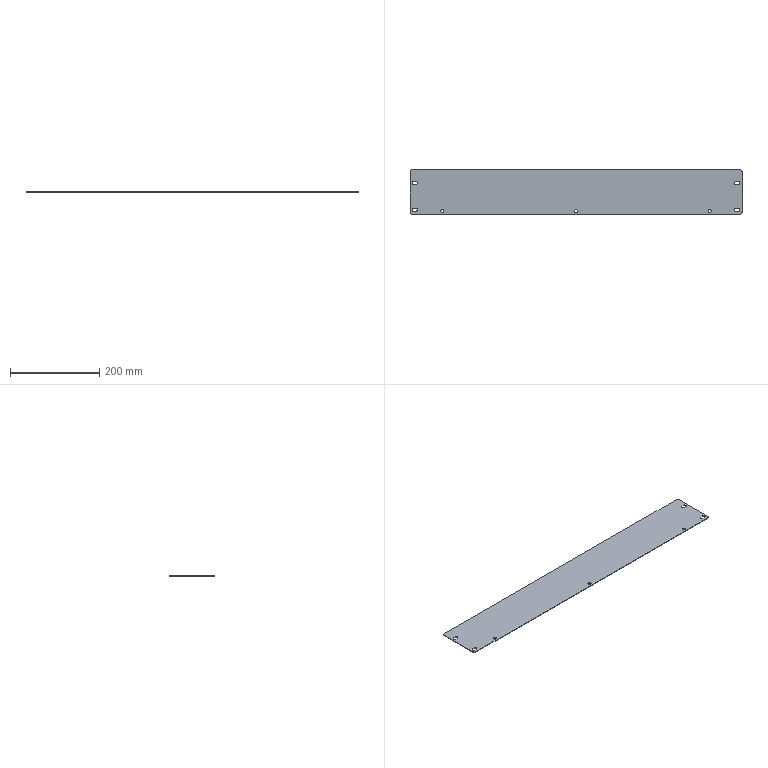Part | SolidWorks | features EdgeFlange 2, Fillet 1, FlatPattern 1, HoleWzd 1, ICE 1, SMBaseFlange 1, SheetMetal 1 | 1 solid | 36 faces | box 745 x 100 x 1.2 mm | volume 88883 mm3 | cylinder 22 | plane 14 | commonest cylinder face diameters 7 x18 10 x4
STEP:
#1=CARTESIAN_POINT('',(303.5,-43.,0.));
#2=VERTEX_POINT('',#1);
#3=CARTESIAN_POINT('',(296.5,-43.,0.));
#4=VERTEX_POINT('',#3);
#5=CARTESIAN_POINT('',(300.,-43.,0.));
#6=DIRECTION('',(0.,0.,-1.));
#7=DIRECTION('',(-1.,0.,0.));
#8=AXIS2_PLACEMENT_3D('',#5,#6,#7);
#9=CIRCLE('',#8,3.5);
#10=EDGE_CURVE('',#2,#4,#9,.T.);
#11=ORIENTED_EDGE('',*,*,#10,.F.);
#12=CARTESIAN_POINT('',(303.5,-43.,-1.2));
#13=VERTEX_POINT('',#12);
#14=CARTESIAN_POINT('',(303.5,-43.,-1.2));
#15=DIRECTION('',(0.,0.,-1.));
#16=VECTOR('',#15,1000.);
#17=LINE('',#14,#16);
#18=EDGE_CURVE('',#2,#13,#17,.T.);
#19=ORIENTED_EDGE('',*,*,#18,.T.);
#20=CARTESIAN_POINT('',(296.5,-43.,-1.2));
#21=VERTEX_POINT('',#20);
#22=CARTESIAN_POINT('',(300.,-43.,-1.2));
#23=DIRECTION('',(0.,0.,-1.));
#24=DIRECTION('',(-1.,0.,0.));
#25=AXIS2_PLACEMENT_3D('',#22,#23,#24);
#26=CIRCLE('',#25,3.5);
#27=EDGE_CURVE('',#13,#21,#26,.T.);
#28=ORIENTED_EDGE('',*,*,#27,.T.);
#29=CARTESIAN_POINT('',(296.5,-43.,-1.2));
#30=DIRECTION('',(0.,0.,-1.));
#31=VECTOR('',#30,1000.);
#32=LINE('',#29,#31);
#33=EDGE_CURVE('',#4,#21,#32,.T.);
#34=ORIENTED_EDGE('',*,*,#33,.F.);
#35=EDGE_LOOP('',(#11,#19,#28,#34));
#36=FACE_OUTER_BOUND('',#35,.T.);
#37=CARTESIAN_POINT('',(300.,-43.,-1.2));
#38=DIRECTION('',(0.,0.,-1.));
#39=DIRECTION('',(-1.,0.,0.));
#40=AXIS2_PLACEMENT_3D('',#37,#38,#39);
#41=CYLINDRICAL_SURFACE('',#40,3.5);
#42=ADVANCED_FACE('',(#36),#41,.F.);
#43=CARTESIAN_POINT('',(3.5,-43.,0.));
#44=VERTEX_POINT('',#43);
#45=CARTESIAN_POINT('',(-3.5,-43.,0.));
#46=VERTEX_POINT('',#45);
#47=CARTESIAN_POINT('',(0.,-43.,0.));
#48=DIRECTION('',(0.,0.,-1.));
#49=DIRECTION('',(-1.,0.,0.));
#50=AXIS2_PLACEMENT_3D('',#47,#48,#49);
#51=CIRCLE('',#50,3.5);
#52=EDGE_CURVE('',#44,#46,#51,.T.);
#53=ORIENTED_EDGE('',*,*,#52,.F.);
#54=CARTESIAN_POINT('',(3.5,-43.,-1.2));
#55=VERTEX_POINT('',#54);
#56=CARTESIAN_POINT('',(3.5,-43.,-1.2));
#57=DIRECTION('',(0.,0.,-1.));
#58=VECTOR('',#57,1000.);
#59=LINE('',#56,#58);
#60=EDGE_CURVE('',#44,#55,#59,.T.);
#61=ORIENTED_EDGE('',*,*,#60,.T.);
#62=CARTESIAN_POINT('',(-3.5,-43.,-1.2));
#63=VERTEX_POINT('',#62);
#64=CARTESIAN_POINT('',(0.,-43.,-1.2));
#65=DIRECTION('',(0.,0.,-1.));
#66=DIRECTION('',(-1.,0.,0.));
#67=AXIS2_PLACEMENT_3D('',#64,#65,#66);
#68=CIRCLE('',#67,3.5);
#69=EDGE_CURVE('',#55,#63,#68,.T.);
#70=ORIENTED_EDGE('',*,*,#69,.T.);
#71=CARTESIAN_POINT('',(-3.5,-43.,-1.2));
#72=DIRECTION('',(0.,0.,-1.));
#73=VECTOR('',#72,1000.);
#74=LINE('',#71,#73);
#75=EDGE_CURVE('',#46,#63,#74,.T.);
#76=ORIENTED_EDGE('',*,*,#75,.F.);
#77=EDGE_LOOP('',(#53,#61,#70,#76));
#78=FACE_OUTER_BOUND('',#77,.T.);
#79=CARTESIAN_POINT('',(0.,-43.,-1.2));
#80=DIRECTION('',(0.,0.,-1.));
#81=DIRECTION('',(-1.,0.,0.));
#82=AXIS2_PLACEMENT_3D('',#79,#80,#81);
#83=CYLINDRICAL_SURFACE('',#82,3.5);
#84=ADVANCED_FACE('',(#78),#83,.F.);
#85=CARTESIAN_POINT('',(-296.5,-43.,0.));
#86=VERTEX_POINT('',#85);
#87=CARTESIAN_POINT('',(-303.5,-43.,0.));
#88=VERTEX_POINT('',#87);
#89=CARTESIAN_POINT('',(-300.,-43.,0.));
#90=DIRECTION('',(0.,0.,-1.));
#91=DIRECTION('',(-1.,0.,0.));
#92=AXIS2_PLACEMENT_3D('',#89,#90,#91);
#93=CIRCLE('',#92,3.5);
#94=EDGE_CURVE('',#86,#88,#93,.T.);
#95=ORIENTED_EDGE('',*,*,#94,.F.);
#96=CARTESIAN_POINT('',(-296.5,-43.,-1.2));
#97=VERTEX_POINT('',#96);
#98=CARTESIAN_POINT('',(-296.5,-43.,-1.2));
#99=DIRECTION('',(0.,0.,-1.));
#100=VECTOR('',#99,1000.);
#101=LINE('',#98,#100);
#102=EDGE_CURVE('',#86,#97,#101,.T.);
#103=ORIENTED_EDGE('',*,*,#102,.T.);
#104=CARTESIAN_POINT('',(-303.5,-43.,-1.2));
#105=VERTEX_POINT('',#104);
#106=CARTESIAN_POINT('',(-300.,-43.,-1.2));
#107=DIRECTION('',(0.,0.,-1.));
#108=DIRECTION('',(-1.,0.,0.));
#109=AXIS2_PLACEMENT_3D('',#106,#107,#108);
#110=CIRCLE('',#109,3.5);
#111=EDGE_CURVE('',#97,#105,#110,.T.);
#112=ORIENTED_EDGE('',*,*,#111,.T.);
#113=CARTESIAN_POINT('',(-303.5,-43.,-1.2));
#114=DIRECTION('',(0.,0.,-1.));
#115=VECTOR('',#114,1000.);
#116=LINE('',#113,#115);
#117=EDGE_CURVE('',#88,#105,#116,.T.);
#118=ORIENTED_EDGE('',*,*,#117,.F.);
#119=EDGE_LOOP('',(#95,#103,#112,#118));
#120=FACE_OUTER_BOUND('',#119,.T.);
#121=CARTESIAN_POINT('',(-300.,-43.,-1.2));
#122=DIRECTION('',(0.,0.,-1.));
#123=DIRECTION('',(-1.,0.,0.));
#124=AXIS2_PLACEMENT_3D('',#121,#122,#123);
#125=CYLINDRICAL_SURFACE('',#124,3.5);
#126=ADVANCED_FACE('',(#120),#125,.F.);
#127=CARTESIAN_POINT('',(359.5,-36.5,0.));
#128=VERTEX_POINT('',#127);
#129=CARTESIAN_POINT('',(356.,-40.,0.));
#130=VERTEX_POINT('',#129);
#131=CARTESIAN_POINT('',(359.5,-40.,0.));
#132=DIRECTION('',(0.,0.,1.));
#133=DIRECTION('',(1.,0.,0.));
#134=AXIS2_PLACEMENT_3D('',#131,#132,#133);
#135=CIRCLE('',#134,3.5);
#136=EDGE_CURVE('',#128,#130,#135,.T.);
#137=ORIENTED_EDGE('',*,*,#136,.T.);
#138=CARTESIAN_POINT('',(356.,-40.,-1.2));
#139=VERTEX_POINT('',#138);
#140=CARTESIAN_POINT('',(356.,-40.,8.8));
#141=DIRECTION('',(0.,0.,-1.));
#142=VECTOR('',#141,1000.);
#143=LINE('',#140,#142);
#144=EDGE_CURVE('',#130,#139,#143,.T.);
#145=ORIENTED_EDGE('',*,*,#144,.T.);
#146=CARTESIAN_POINT('',(359.5,-36.5,-1.2));
#147=VERTEX_POINT('',#146);
#148=CARTESIAN_POINT('',(359.5,-40.,-1.2));
#149=DIRECTION('',(0.,0.,-1.));
#150=DIRECTION('',(-1.,0.,0.));
#151=AXIS2_PLACEMENT_3D('',#148,#149,#150);
#152=CIRCLE('',#151,3.5);
#153=EDGE_CURVE('',#139,#147,#152,.T.);
#154=ORIENTED_EDGE('',*,*,#153,.T.);
#155=CARTESIAN_POINT('',(359.5,-36.5,8.8));
#156=DIRECTION('',(0.,0.,-1.));
#157=VECTOR('',#156,1000.);
#158=LINE('',#155,#157);
#159=EDGE_CURVE('',#128,#147,#158,.T.);
#160=ORIENTED_EDGE('',*,*,#159,.F.);
#161=EDGE_LOOP('',(#137,#145,#154,#160));
#162=FACE_OUTER_BOUND('',#161,.T.);
#163=CARTESIAN_POINT('',(359.5,-40.,8.8));
#164=DIRECTION('',(0.,0.,-1.));
#165=DIRECTION('',(-1.,0.,0.));
#166=AXIS2_PLACEMENT_3D('',#163,#164,#165);
#167=CYLINDRICAL_SURFACE('',#166,3.5);
#168=ADVANCED_FACE('',(#162),#167,.F.);
#169=CARTESIAN_POINT('',(-364.5,23.5,0.));
#170=VERTEX_POINT('',#169);
#171=CARTESIAN_POINT('',(-368.,20.,0.));
#172=VERTEX_POINT('',#171);
#173=CARTESIAN_POINT('',(-364.5,20.,0.));
#174=DIRECTION('',(0.,0.,1.));
#175=DIRECTION('',(1.,0.,0.));
#176=AXIS2_PLACEMENT_3D('',#173,#174,#175);
#177=CIRCLE('',#176,3.5);
#178=EDGE_CURVE('',#170,#172,#177,.T.);
#179=ORIENTED_EDGE('',*,*,#178,.T.);
#180=CARTESIAN_POINT('',(-368.,20.,-1.2));
#181=VERTEX_POINT('',#180);
#182=CARTESIAN_POINT('',(-368.,20.,8.8));
#183=DIRECTION('',(0.,0.,-1.));
#184=VECTOR('',#183,1000.);
#185=LINE('',#182,#184);
#186=EDGE_CURVE('',#172,#181,#185,.T.);
#187=ORIENTED_EDGE('',*,*,#186,.T.);
#188=CARTESIAN_POINT('',(-364.5,23.5,-1.2));
#189=VERTEX_POINT('',#188);
#190=CARTESIAN_POINT('',(-364.5,20.,-1.2));
#191=DIRECTION('',(0.,0.,-1.));
#192=DIRECTION('',(1.,0.,0.));
#193=AXIS2_PLACEMENT_3D('',#190,#191,#192);
#194=CIRCLE('',#193,3.5);
#195=EDGE_CURVE('',#181,#189,#194,.T.);
#196=ORIENTED_EDGE('',*,*,#195,.T.);
#197=CARTESIAN_POINT('',(-364.5,23.5,8.8));
#198=DIRECTION('',(0.,0.,-1.));
#199=VECTOR('',#198,1000.);
#200=LINE('',#197,#199);
#201=EDGE_CURVE('',#170,#189,#200,.T.);
#202=ORIENTED_EDGE('',*,*,#201,.F.);
#203=EDGE_LOOP('',(#179,#187,#196,#202));
#204=FACE_OUTER_BOUND('',#203,.T.);
#205=CARTESIAN_POINT('',(-364.5,20.,8.8));
#206=DIRECTION('',(0.,0.,-1.));
#207=DIRECTION('',(-1.,0.,0.));
#208=AXIS2_PLACEMENT_3D('',#205,#206,#207);
#209=CYLINDRICAL_SURFACE('',#208,3.5);
#210=ADVANCED_FACE('',(#204),#209,.F.);
#211=CARTESIAN_POINT('',(-364.5,-36.5,0.));
#212=VERTEX_POINT('',#211);
#213=CARTESIAN_POINT('',(-368.,-40.,0.));
#214=VERTEX_POINT('',#213);
#215=CARTESIAN_POINT('',(-364.5,-40.,0.));
#216=DIRECTION('',(0.,0.,1.));
#217=DIRECTION('',(1.,0.,0.));
#218=AXIS2_PLACEMENT_3D('',#215,#216,#217);
#219=CIRCLE('',#218,3.5);
#220=EDGE_CURVE('',#212,#214,#219,.T.);
#221=ORIENTED_EDGE('',*,*,#220,.T.);
#222=CARTESIAN_POINT('',(-368.,-40.,-1.2));
#223=VERTEX_POINT('',#222);
#224=CARTESIAN_POINT('',(-368.,-40.,8.8));
#225=DIRECTION('',(0.,0.,-1.));
#226=VECTOR('',#225,1000.);
#227=LINE('',#224,#226);
#228=EDGE_CURVE('',#214,#223,#227,.T.);
#229=ORIENTED_EDGE('',*,*,#228,.T.);
#230=CARTESIAN_POINT('',(-364.5,-36.5,-1.2));
#231=VERTEX_POINT('',#230);
#232=CARTESIAN_POINT('',(-364.5,-40.,-1.2));
#233=DIRECTION('',(0.,0.,-1.));
#234=DIRECTION('',(1.,0.,0.));
#235=AXIS2_PLACEMENT_3D('',#232,#233,#234);
#236=CIRCLE('',#235,3.5);
#237=EDGE_CURVE('',#223,#231,#236,.T.);
#238=ORIENTED_EDGE('',*,*,#237,.T.);
#239=CARTESIAN_POINT('',(-364.5,-36.5,8.8));
#240=DIRECTION('',(0.,0.,-1.));
#241=VECTOR('',#240,1000.);
#242=LINE('',#239,#241);
#243=EDGE_CURVE('',#212,#231,#242,.T.);
#244=ORIENTED_EDGE('',*,*,#243,.F.);
#245=EDGE_LOOP('',(#221,#229,#238,#244));
#246=FACE_OUTER_BOUND('',#245,.T.);
#247=CARTESIAN_POINT('',(-364.5,-40.,8.8));
#248=DIRECTION('',(0.,0.,-1.));
#249=DIRECTION('',(-1.,0.,0.));
#250=AXIS2_PLACEMENT_3D('',#247,#248,#249);
#251=CYLINDRICAL_SURFACE('',#250,3.5);
#252=ADVANCED_FACE('',(#246),#251,.F.);
#253=CARTESIAN_POINT('',(359.5,23.5,0.));
#254=VERTEX_POINT('',#253);
#255=CARTESIAN_POINT('',(356.,20.,0.));
#256=VERTEX_POINT('',#255);
#257=CARTESIAN_POINT('',(359.5,20.,0.));
#258=DIRECTION('',(0.,0.,1.));
#259=DIRECTION('',(1.,0.,0.));
#260=AXIS2_PLACEMENT_3D('',#257,#258,#259);
#261=CIRCLE('',#260,3.5);
#262=EDGE_CURVE('',#254,#256,#261,.T.);
#263=ORIENTED_EDGE('',*,*,#262,.T.);
#264=CARTESIAN_POINT('',(356.,20.,-1.2));
#265=VERTEX_POINT('',#264);
#266=CARTESIAN_POINT('',(356.,20.,8.8));
#267=DIRECTION('',(0.,0.,-1.));
#268=VECTOR('',#267,1000.);
#269=LINE('',#266,#268);
#270=EDGE_CURVE('',#256,#265,#269,.T.);
#271=ORIENTED_EDGE('',*,*,#270,.T.);
#272=CARTESIAN_POINT('',(359.5,23.5,-1.2));
#273=VERTEX_POINT('',#272);
#274=CARTESIAN_POINT('',(359.5,20.,-1.2));
#275=DIRECTION('',(0.,0.,-1.));
#276=DIRECTION('',(-1.,0.,0.));
#277=AXIS2_PLACEMENT_3D('',#274,#275,#276);
#278=CIRCLE('',#277,3.5);
#279=EDGE_CURVE('',#265,#273,#278,.T.);
#280=ORIENTED_EDGE('',*,*,#279,.T.);
#281=CARTESIAN_POINT('',(359.5,23.5,8.8));
#282=DIRECTION('',(0.,0.,-1.));
#283=VECTOR('',#282,1000.);
#284=LINE('',#281,#283);
#285=EDGE_CURVE('',#254,#273,#284,.T.);
#286=ORIENTED_EDGE('',*,*,#285,.F.);
#287=EDGE_LOOP('',(#263,#271,#280,#286));
#288=FACE_OUTER_BOUND('',#287,.T.);
#289=CARTESIAN_POINT('',(359.5,20.,8.8));
#290=DIRECTION('',(0.,0.,-1.));
#291=DIRECTION('',(-1.,0.,0.));
#292=AXIS2_PLACEMENT_3D('',#289,#290,#291);
#293=CYLINDRICAL_SURFACE('',#292,3.5);
#294=ADVANCED_FACE('',(#288),#293,.F.);
#295=CARTESIAN_POINT('',(372.5,-45.,0.));
#296=VERTEX_POINT('',#295);
#297=CARTESIAN_POINT('',(372.5,45.,0.));
#298=VERTEX_POINT('',#297);
#299=CARTESIAN_POINT('',(372.5,50.,0.));
#300=DIRECTION('',(0.,1.,0.));
#301=VECTOR('',#300,1000.);
#302=LINE('',#299,#301);
#303=EDGE_CURVE('',#296,#298,#302,.T.);
#304=ORIENTED_EDGE('',*,*,#303,.F.);
#305=CARTESIAN_POINT('',(372.5,-45.,-1.2));
#306=VERTEX_POINT('',#305);
#307=CARTESIAN_POINT('',(372.5,-45.,-1.2));
#308=DIRECTION('',(0.,0.,-1.));
#309=VECTOR('',#308,1000.);
#310=LINE('',#307,#309);
#311=EDGE_CURVE('',#296,#306,#310,.T.);
#312=ORIENTED_EDGE('',*,*,#311,.T.);
#313=CARTESIAN_POINT('',(372.5,45.,-1.2));
#314=VERTEX_POINT('',#313);
#315=CARTESIAN_POINT('',(372.5,50.,-1.2));
#316=DIRECTION('',(0.,1.,0.));
#317=VECTOR('',#316,1000.);
#318=LINE('',#315,#317);
#319=EDGE_CURVE('',#306,#314,#318,.T.);
#320=ORIENTED_EDGE('',*,*,#319,.T.);
#321=CARTESIAN_POINT('',(372.5,45.,-1.2));
#322=DIRECTION('',(0.,0.,1.));
#323=VECTOR('',#322,1000.);
#324=LINE('',#321,#323);
#325=EDGE_CURVE('',#314,#298,#324,.T.);
#326=ORIENTED_EDGE('',*,*,#325,.T.);
#327=EDGE_LOOP('',(#304,#312,#320,#326));
#328=FACE_OUTER_BOUND('',#327,.T.);
#329=CARTESIAN_POINT('',(372.5,50.,-1.2));
#330=DIRECTION('',(1.,0.,0.));
#331=DIRECTION('',(0.,0.,-1.));
#332=AXIS2_PLACEMENT_3D('',#329,#330,#331);
#333=PLANE('',#332);
#334=ADVANCED_FACE('',(#328),#333,.T.);
#335=CARTESIAN_POINT('',(-367.5,-50.,0.));
#336=VERTEX_POINT('',#335);
#337=CARTESIAN_POINT('',(367.5,-50.,0.));
#338=VERTEX_POINT('',#337);
#339=CARTESIAN_POINT('',(-372.5,-50.,0.));
#340=DIRECTION('',(1.,0.,0.));
#341=VECTOR('',#340,1000.);
#342=LINE('',#339,#341);
#343=EDGE_CURVE('',#336,#338,#342,.T.);
#344=ORIENTED_EDGE('',*,*,#343,.F.);
#345=CARTESIAN_POINT('',(-367.5,-50.,-1.2));
#346=VERTEX_POINT('',#345);
#347=CARTESIAN_POINT('',(-367.5,-50.,-1.2));
#348=DIRECTION('',(0.,0.,-1.));
#349=VECTOR('',#348,1000.);
#350=LINE('',#347,#349);
#351=EDGE_CURVE('',#336,#346,#350,.T.);
#352=ORIENTED_EDGE('',*,*,#351,.T.);
#353=CARTESIAN_POINT('',(367.5,-50.,-1.2));
#354=VERTEX_POINT('',#353);
#355=CARTESIAN_POINT('',(-372.5,-50.,-1.2));
#356=DIRECTION('',(1.,0.,0.));
#357=VECTOR('',#356,1000.);
#358=LINE('',#355,#357);
#359=EDGE_CURVE('',#346,#354,#358,.T.);
#360=ORIENTED_EDGE('',*,*,#359,.T.);
#361=CARTESIAN_POINT('',(367.5,-50.,-1.2));
#362=DIRECTION('',(0.,0.,1.));
#363=VECTOR('',#362,1000.);
#364=LINE('',#361,#363);
#365=EDGE_CURVE('',#354,#338,#364,.T.);
#366=ORIENTED_EDGE('',*,*,#365,.T.);
#367=EDGE_LOOP('',(#344,#352,#360,#366));
#368=FACE_OUTER_BOUND('',#367,.T.);
#369=CARTESIAN_POINT('',(-372.5,-50.,-1.2));
#370=DIRECTION('',(0.,-1.,0.));
#371=DIRECTION('',(0.,0.,-1.));
#372=AXIS2_PLACEMENT_3D('',#369,#370,#371);
#373=PLANE('',#372);
#374=ADVANCED_FACE('',(#368),#373,.T.);
#375=CARTESIAN_POINT('',(-372.5,45.,0.));
#376=VERTEX_POINT('',#375);
#377=CARTESIAN_POINT('',(-372.5,-45.,0.));
#378=VERTEX_POINT('',#377);
#379=CARTESIAN_POINT('',(-372.5,50.,0.));
#380=DIRECTION('',(0.,-1.,0.));
#381=VECTOR('',#380,1000.);
#382=LINE('',#379,#381);
#383=EDGE_CURVE('',#376,#378,#382,.T.);
#384=ORIENTED_EDGE('',*,*,#383,.F.);
#385=CARTESIAN_POINT('',(-372.5,45.,-1.2));
#386=VERTEX_POINT('',#385);
#387=CARTESIAN_POINT('',(-372.5,45.,-1.2));
#388=DIRECTION('',(0.,0.,-1.));
#389=VECTOR('',#388,1000.);
#390=LINE('',#387,#389);
#391=EDGE_CURVE('',#376,#386,#390,.T.);
#392=ORIENTED_EDGE('',*,*,#391,.T.);
#393=CARTESIAN_POINT('',(-372.5,-45.,-1.2));
#394=VERTEX_POINT('',#393);
#395=CARTESIAN_POINT('',(-372.5,50.,-1.2));
#396=DIRECTION('',(0.,-1.,0.));
#397=VECTOR('',#396,1000.);
#398=LINE('',#395,#397);
#399=EDGE_CURVE('',#386,#394,#398,.T.);
#400=ORIENTED_EDGE('',*,*,#399,.T.);
#401=CARTESIAN_POINT('',(-372.5,-45.,-1.2));
#402=DIRECTION('',(0.,0.,1.));
#403=VECTOR('',#402,1000.);
#404=LINE('',#401,#403);
#405=EDGE_CURVE('',#394,#378,#404,.T.);
#406=ORIENTED_EDGE('',*,*,#405,.T.);
#407=EDGE_LOOP('',(#384,#392,#400,#406));
#408=FACE_OUTER_BOUND('',#407,.T.);
#409=CARTESIAN_POINT('',(-372.5,50.,-1.2));
#410=DIRECTION('',(-1.,0.,0.));
#411=DIRECTION('',(0.,0.,1.));
#412=AXIS2_PLACEMENT_3D('',#409,#410,#411);
#413=PLANE('',#412);
#414=ADVANCED_FACE('',(#408),#413,.T.);
#415=CARTESIAN_POINT('',(367.5,50.,-1.2));
#416=VERTEX_POINT('',#415);
#417=CARTESIAN_POINT('',(-367.5,50.,-1.2));
#418=VERTEX_POINT('',#417);
#419=CARTESIAN_POINT('',(-372.5,50.,-1.2));
#420=DIRECTION('',(-1.,0.,0.));
#421=VECTOR('',#420,1000.);
#422=LINE('',#419,#421);
#423=EDGE_CURVE('',#416,#418,#422,.T.);
#424=ORIENTED_EDGE('',*,*,#423,.T.);
#425=CARTESIAN_POINT('',(-367.5,50.,0.));
#426=VERTEX_POINT('',#425);
#427=CARTESIAN_POINT('',(-367.5,50.,-1.2));
#428=DIRECTION('',(0.,0.,1.));
#429=VECTOR('',#428,1000.);
#430=LINE('',#427,#429);
#431=EDGE_CURVE('',#418,#426,#430,.T.);
#432=ORIENTED_EDGE('',*,*,#431,.T.);
#433=CARTESIAN_POINT('',(367.5,50.,0.));
#434=VERTEX_POINT('',#433);
#435=CARTESIAN_POINT('',(-372.5,50.,0.));
#436=DIRECTION('',(-1.,0.,0.));
#437=VECTOR('',#436,1000.);
#438=LINE('',#435,#437);
#439=EDGE_CURVE('',#434,#426,#438,.T.);
#440=ORIENTED_EDGE('',*,*,#439,.F.);
#441=CARTESIAN_POINT('',(367.5,50.,-1.2));
#442=DIRECTION('',(0.,0.,-1.));
#443=VECTOR('',#442,1000.);
#444=LINE('',#441,#443);
#445=EDGE_CURVE('',#434,#416,#444,.T.);
#446=ORIENTED_EDGE('',*,*,#445,.T.);
#447=EDGE_LOOP('',(#424,#432,#440,#446));
#448=FACE_OUTER_BOUND('',#447,.T.);
#449=CARTESIAN_POINT('',(-372.5,50.,-1.2));
#450=DIRECTION('',(0.,1.,0.));
#451=DIRECTION('',(0.,0.,1.));
#452=AXIS2_PLACEMENT_3D('',#449,#450,#451);
#453=PLANE('',#452);
#454=ADVANCED_FACE('',(#448),#453,.T.);
#455=CARTESIAN_POINT('',(300.,-43.,-1.2));
#456=DIRECTION('',(0.,0.,-1.));
#457=DIRECTION('',(-1.,0.,0.));
#458=AXIS2_PLACEMENT_3D('',#455,#456,#457);
#459=CIRCLE('',#458,3.5);
#460=EDGE_CURVE('',#21,#13,#459,.T.);
#461=ORIENTED_EDGE('',*,*,#460,.F.);
#462=ORIENTED_EDGE('',*,*,#27,.F.);
#463=EDGE_LOOP('',(#461,#462));
#464=FACE_BOUND('',#463,.T.);
#465=CARTESIAN_POINT('',(0.,-43.,-1.2));
#466=DIRECTION('',(0.,0.,-1.));
#467=DIRECTION('',(-1.,0.,0.));
#468=AXIS2_PLACEMENT_3D('',#465,#466,#467);
#469=CIRCLE('',#468,3.5);
#470=EDGE_CURVE('',#63,#55,#469,.T.);
#471=ORIENTED_EDGE('',*,*,#470,.F.);
#472=ORIENTED_EDGE('',*,*,#69,.F.);
#473=EDGE_LOOP('',(#471,#472));
#474=FACE_BOUND('',#473,.T.);
#475=CARTESIAN_POINT('',(-300.,-43.,-1.2));
#476=DIRECTION('',(0.,0.,-1.));
#477=DIRECTION('',(-1.,0.,0.));
#478=AXIS2_PLACEMENT_3D('',#475,#476,#477);
#479=CIRCLE('',#478,3.5);
#480=EDGE_CURVE('',#105,#97,#479,.T.);
#481=ORIENTED_EDGE('',*,*,#480,.F.);
#482=ORIENTED_EDGE('',*,*,#111,.F.);
#483=EDGE_LOOP('',(#481,#482));
#484=FACE_BOUND('',#483,.T.);
#485=CARTESIAN_POINT('',(364.5,-43.5,-1.2));
#486=VERTEX_POINT('',#485);
#487=CARTESIAN_POINT('',(359.5,-43.5,-1.2));
#488=VERTEX_POINT('',#487);
#489=CARTESIAN_POINT('',(364.5,-43.5,-1.2));
#490=DIRECTION('',(-1.,0.,0.));
#491=VECTOR('',#490,1000.);
#492=LINE('',#489,#491);
#493=EDGE_CURVE('',#486,#488,#492,.T.);
#494=ORIENTED_EDGE('',*,*,#493,.F.);
#495=CARTESIAN_POINT('',(364.5,-36.5,-1.2));
#496=VERTEX_POINT('',#495);
#497=CARTESIAN_POINT('',(364.5,-40.,-1.2));
#498=DIRECTION('',(0.,0.,-1.));
#499=DIRECTION('',(-1.,0.,0.));
#500=AXIS2_PLACEMENT_3D('',#497,#498,#499);
#501=CIRCLE('',#500,3.5);
#502=EDGE_CURVE('',#496,#486,#501,.T.);
#503=ORIENTED_EDGE('',*,*,#502,.F.);
#504=CARTESIAN_POINT('',(364.5,-36.5,-1.2));
#505=DIRECTION('',(1.,0.,0.));
#506=VECTOR('',#505,1000.);
#507=LINE('',#504,#506);
#508=EDGE_CURVE('',#147,#496,#507,.T.);
#509=ORIENTED_EDGE('',*,*,#508,.F.);
#510=ORIENTED_EDGE('',*,*,#153,.F.);
#511=CARTESIAN_POINT('',(359.5,-40.,-1.2));
#512=DIRECTION('',(0.,0.,-1.));
#513=DIRECTION('',(-1.,0.,0.));
#514=AXIS2_PLACEMENT_3D('',#511,#512,#513);
#515=CIRCLE('',#514,3.5);
#516=EDGE_CURVE('',#488,#139,#515,.T.);
#517=ORIENTED_EDGE('',*,*,#516,.F.);
#518=EDGE_LOOP('',(#494,#503,#509,#510,#517));
#519=FACE_BOUND('',#518,.T.);
#520=CARTESIAN_POINT('',(-359.5,23.5,-1.2));
#521=VERTEX_POINT('',#520);
#522=CARTESIAN_POINT('',(-364.5,23.5,-1.2));
#523=DIRECTION('',(1.,0.,0.));
#524=VECTOR('',#523,1000.);
#525=LINE('',#522,#524);
#526=EDGE_CURVE('',#189,#521,#525,.T.);
#527=ORIENTED_EDGE('',*,*,#526,.F.);
#528=ORIENTED_EDGE('',*,*,#195,.F.);
#529=CARTESIAN_POINT('',(-364.5,16.5,-1.2));
#530=VERTEX_POINT('',#529);
#531=CARTESIAN_POINT('',(-364.5,20.,-1.2));
#532=DIRECTION('',(0.,0.,-1.));
#533=DIRECTION('',(1.,0.,0.));
#534=AXIS2_PLACEMENT_3D('',#531,#532,#533);
#535=CIRCLE('',#534,3.5);
#536=EDGE_CURVE('',#530,#181,#535,.T.);
#537=ORIENTED_EDGE('',*,*,#536,.F.);
#538=CARTESIAN_POINT('',(-359.5,16.5,-1.2));
#539=VERTEX_POINT('',#538);
#540=CARTESIAN_POINT('',(-364.5,16.5,-1.2));
#541=DIRECTION('',(-1.,0.,0.));
#542=VECTOR('',#541,1000.);
#543=LINE('',#540,#542);
#544=EDGE_CURVE('',#539,#530,#543,.T.);
#545=ORIENTED_EDGE('',*,*,#544,.F.);
#546=CARTESIAN_POINT('',(-359.5,20.,-1.2));
#547=DIRECTION('',(0.,0.,-1.));
#548=DIRECTION('',(1.,0.,0.));
#549=AXIS2_PLACEMENT_3D('',#546,#547,#548);
#550=CIRCLE('',#549,3.5);
#551=EDGE_CURVE('',#521,#539,#550,.T.);
#552=ORIENTED_EDGE('',*,*,#551,.F.);
#553=EDGE_LOOP('',(#527,#528,#537,#545,#552));
#554=FACE_BOUND('',#553,.T.);
#555=CARTESIAN_POINT('',(-359.5,-36.5,-1.2));
#556=VERTEX_POINT('',#555);
#557=CARTESIAN_POINT('',(-364.5,-36.5,-1.2));
#558=DIRECTION('',(1.,0.,0.));
#559=VECTOR('',#558,1000.);
#560=LINE('',#557,#559);
#561=EDGE_CURVE('',#231,#556,#560,.T.);
#562=ORIENTED_EDGE('',*,*,#561,.F.);
#563=ORIENTED_EDGE('',*,*,#237,.F.);
#564=CARTESIAN_POINT('',(-364.5,-43.5,-1.2));
#565=VERTEX_POINT('',#564);
#566=CARTESIAN_POINT('',(-364.5,-40.,-1.2));
#567=DIRECTION('',(0.,0.,-1.));
#568=DIRECTION('',(1.,0.,0.));
#569=AXIS2_PLACEMENT_3D('',#566,#567,#568);
#570=CIRCLE('',#569,3.5);
#571=EDGE_CURVE('',#565,#223,#570,.T.);
#572=ORIENTED_EDGE('',*,*,#571,.F.);
#573=CARTESIAN_POINT('',(-359.5,-43.5,-1.2));
#574=VERTEX_POINT('',#573);
#575=CARTESIAN_POINT('',(-364.5,-43.5,-1.2));
#576=DIRECTION('',(-1.,0.,0.));
#577=VECTOR('',#576,1000.);
#578=LINE('',#575,#577);
#579=EDGE_CURVE('',#574,#565,#578,.T.);
#580=ORIENTED_EDGE('',*,*,#579,.F.);
#581=CARTESIAN_POINT('',(-359.5,-40.,-1.2));
#582=DIRECTION('',(0.,0.,-1.));
#583=DIRECTION('',(1.,0.,0.));
#584=AXIS2_PLACEMENT_3D('',#581,#582,#583);
#585=CIRCLE('',#584,3.5);
#586=EDGE_CURVE('',#556,#574,#585,.T.);
#587=ORIENTED_EDGE('',*,*,#586,.F.);
#588=EDGE_LOOP('',(#562,#563,#572,#580,#587));
#589=FACE_BOUND('',#588,.T.);
#590=CARTESIAN_POINT('',(364.5,16.5,-1.2));
#591=VERTEX_POINT('',#590);
#592=CARTESIAN_POINT('',(359.5,16.5,-1.2));
#593=VERTEX_POINT('',#592);
#594=CARTESIAN_POINT('',(364.5,16.5,-1.2));
#595=DIRECTION('',(-1.,0.,0.));
#596=VECTOR('',#595,1000.);
#597=LINE('',#594,#596);
#598=EDGE_CURVE('',#591,#593,#597,.T.);
#599=ORIENTED_EDGE('',*,*,#598,.F.);
#600=CARTESIAN_POINT('',(364.5,23.5,-1.2));
#601=VERTEX_POINT('',#600);
#602=CARTESIAN_POINT('',(364.5,20.,-1.2));
#603=DIRECTION('',(0.,0.,-1.));
#604=DIRECTION('',(-1.,0.,0.));
#605=AXIS2_PLACEMENT_3D('',#602,#603,#604);
#606=CIRCLE('',#605,3.5);
#607=EDGE_CURVE('',#601,#591,#606,.T.);
#608=ORIENTED_EDGE('',*,*,#607,.F.);
#609=CARTESIAN_POINT('',(364.5,23.5,-1.2));
#610=DIRECTION('',(1.,0.,0.));
#611=VECTOR('',#610,1000.);
#612=LINE('',#609,#611);
#613=EDGE_CURVE('',#273,#601,#612,.T.);
#614=ORIENTED_EDGE('',*,*,#613,.F.);
#615=ORIENTED_EDGE('',*,*,#279,.F.);
#616=CARTESIAN_POINT('',(359.5,20.,-1.2));
#617=DIRECTION('',(0.,0.,-1.));
#618=DIRECTION('',(-1.,0.,0.));
#619=AXIS2_PLACEMENT_3D('',#616,#617,#618);
#620=CIRCLE('',#619,3.5);
#621=EDGE_CURVE('',#593,#265,#620,.T.);
#622=ORIENTED_EDGE('',*,*,#621,.F.);
#623=EDGE_LOOP('',(#599,#608,#614,#615,#622));
#624=FACE_BOUND('',#623,.T.);
#625=ORIENTED_EDGE('',*,*,#399,.F.);
#626=CARTESIAN_POINT('',(-367.5,45.,-1.2));
#627=DIRECTION('',(0.,0.,-1.));
#628=DIRECTION('',(1.,0.,0.));
#629=AXIS2_PLACEMENT_3D('',#626,#627,#628);
#630=CIRCLE('',#629,5.);
#631=EDGE_CURVE('',#386,#418,#630,.T.);
#632=ORIENTED_EDGE('',*,*,#631,.T.);
#633=ORIENTED_EDGE('',*,*,#423,.F.);
#634=CARTESIAN_POINT('',(367.5,45.,-1.2));
#635=DIRECTION('',(0.,0.,-1.));
#636=DIRECTION('',(1.,0.,0.));
#637=AXIS2_PLACEMENT_3D('',#634,#635,#636);
#638=CIRCLE('',#637,5.);
#639=EDGE_CURVE('',#416,#314,#638,.T.);
#640=ORIENTED_EDGE('',*,*,#639,.T.);
#641=ORIENTED_EDGE('',*,*,#319,.F.);
#642=CARTESIAN_POINT('',(367.5,-45.,-1.2));
#643=DIRECTION('',(0.,0.,-1.));
#644=DIRECTION('',(1.,0.,0.));
#645=AXIS2_PLACEMENT_3D('',#642,#643,#644);
#646=CIRCLE('',#645,5.);
#647=EDGE_CURVE('',#306,#354,#646,.T.);
#648=ORIENTED_EDGE('',*,*,#647,.T.);
#649=ORIENTED_EDGE('',*,*,#359,.F.);
#650=CARTESIAN_POINT('',(-367.5,-45.,-1.2));
#651=DIRECTION('',(0.,0.,-1.));
#652=DIRECTION('',(1.,0.,0.));
#653=AXIS2_PLACEMENT_3D('',#650,#651,#652);
#654=CIRCLE('',#653,5.);
#655=EDGE_CURVE('',#346,#394,#654,.T.);
#656=ORIENTED_EDGE('',*,*,#655,.T.);
#657=EDGE_LOOP('',(#625,#632,#633,#640,#641,#648,#649,#656));
#658=FACE_OUTER_BOUND('',#657,.T.);
#659=CARTESIAN_POINT('',(0.,0.,-1.2));
#660=DIRECTION('',(0.,0.,1.));
#661=DIRECTION('',(1.,0.,0.));
#662=AXIS2_PLACEMENT_3D('',#659,#660,#661);
#663=PLANE('',#662);
#664=ADVANCED_FACE('',(#464,#474,#484,#519,#554,#589,#624,#658),#663,.F.);
#665=CARTESIAN_POINT('',(300.,-43.,0.));
#666=DIRECTION('',(0.,0.,-1.));
#667=DIRECTION('',(-1.,0.,0.));
#668=AXIS2_PLACEMENT_3D('',#665,#666,#667);
#669=CIRCLE('',#668,3.5);
#670=EDGE_CURVE('',#4,#2,#669,.T.);
#671=ORIENTED_EDGE('',*,*,#670,.T.);
#672=ORIENTED_EDGE('',*,*,#10,.T.);
#673=EDGE_LOOP('',(#671,#672));
#674=FACE_BOUND('',#673,.T.);
#675=CARTESIAN_POINT('',(0.,-43.,0.));
#676=DIRECTION('',(0.,0.,-1.));
#677=DIRECTION('',(-1.,0.,0.));
#678=AXIS2_PLACEMENT_3D('',#675,#676,#677);
#679=CIRCLE('',#678,3.5);
#680=EDGE_CURVE('',#46,#44,#679,.T.);
#681=ORIENTED_EDGE('',*,*,#680,.T.);
#682=ORIENTED_EDGE('',*,*,#52,.T.);
#683=EDGE_LOOP('',(#681,#682));
#684=FACE_BOUND('',#683,.T.);
#685=CARTESIAN_POINT('',(-300.,-43.,0.));
#686=DIRECTION('',(0.,0.,-1.));
#687=DIRECTION('',(-1.,0.,0.));
#688=AXIS2_PLACEMENT_3D('',#685,#686,#687);
#689=CIRCLE('',#688,3.5);
#690=EDGE_CURVE('',#88,#86,#689,.T.);
#691=ORIENTED_EDGE('',*,*,#690,.T.);
#692=ORIENTED_EDGE('',*,*,#94,.T.);
#693=EDGE_LOOP('',(#691,#692));
#694=FACE_BOUND('',#693,.T.);
#695=CARTESIAN_POINT('',(364.5,-43.5,0.));
#696=VERTEX_POINT('',#695);
#697=CARTESIAN_POINT('',(364.5,-36.5,0.));
#698=VERTEX_POINT('',#697);
#699=CARTESIAN_POINT('',(364.5,-40.,0.));
#700=DIRECTION('',(0.,0.,1.));
#701=DIRECTION('',(1.,0.,0.));
#702=AXIS2_PLACEMENT_3D('',#699,#700,#701);
#703=CIRCLE('',#702,3.5);
#704=EDGE_CURVE('',#696,#698,#703,.T.);
#705=ORIENTED_EDGE('',*,*,#704,.F.);
#706=CARTESIAN_POINT('',(359.5,-43.5,0.));
#707=VERTEX_POINT('',#706);
#708=CARTESIAN_POINT('',(0.,-43.5,0.));
#709=DIRECTION('',(1.,0.,0.));
#710=VECTOR('',#709,1000.);
#711=LINE('',#708,#710);
#712=EDGE_CURVE('',#707,#696,#711,.T.);
#713=ORIENTED_EDGE('',*,*,#712,.F.);
#714=CARTESIAN_POINT('',(359.5,-40.,0.));
#715=DIRECTION('',(0.,0.,1.));
#716=DIRECTION('',(1.,0.,0.));
#717=AXIS2_PLACEMENT_3D('',#714,#715,#716);
#718=CIRCLE('',#717,3.5);
#719=EDGE_CURVE('',#130,#707,#718,.T.);
#720=ORIENTED_EDGE('',*,*,#719,.F.);
#721=ORIENTED_EDGE('',*,*,#136,.F.);
#722=CARTESIAN_POINT('',(0.,-36.5,0.));
#723=DIRECTION('',(-1.,0.,0.));
#724=VECTOR('',#723,1000.);
#725=LINE('',#722,#724);
#726=EDGE_CURVE('',#698,#128,#725,.T.);
#727=ORIENTED_EDGE('',*,*,#726,.F.);
#728=EDGE_LOOP('',(#705,#713,#720,#721,#727));
#729=FACE_BOUND('',#728,.T.);
#730=ORIENTED_EDGE('',*,*,#178,.F.);
#731=CARTESIAN_POINT('',(-359.5,23.5,0.));
#732=VERTEX_POINT('',#731);
#733=CARTESIAN_POINT('',(0.,23.5,0.));
#734=DIRECTION('',(-1.,0.,0.));
#735=VECTOR('',#734,1000.);
#736=LINE('',#733,#735);
#737=EDGE_CURVE('',#732,#170,#736,.T.);
#738=ORIENTED_EDGE('',*,*,#737,.F.);
#739=CARTESIAN_POINT('',(-359.5,16.5,0.));
#740=VERTEX_POINT('',#739);
#741=CARTESIAN_POINT('',(-359.5,20.,0.));
#742=DIRECTION('',(0.,0.,1.));
#743=DIRECTION('',(1.,0.,0.));
#744=AXIS2_PLACEMENT_3D('',#741,#742,#743);
#745=CIRCLE('',#744,3.5);
#746=EDGE_CURVE('',#740,#732,#745,.T.);
#747=ORIENTED_EDGE('',*,*,#746,.F.);
#748=CARTESIAN_POINT('',(-364.5,16.5,0.));
#749=VERTEX_POINT('',#748);
#750=CARTESIAN_POINT('',(0.,16.5,0.));
#751=DIRECTION('',(1.,0.,0.));
#752=VECTOR('',#751,1000.);
#753=LINE('',#750,#752);
#754=EDGE_CURVE('',#749,#740,#753,.T.);
#755=ORIENTED_EDGE('',*,*,#754,.F.);
#756=CARTESIAN_POINT('',(-364.5,20.,0.));
#757=DIRECTION('',(0.,0.,1.));
#758=DIRECTION('',(1.,0.,0.));
#759=AXIS2_PLACEMENT_3D('',#756,#757,#758);
#760=CIRCLE('',#759,3.5);
#761=EDGE_CURVE('',#172,#749,#760,.T.);
#762=ORIENTED_EDGE('',*,*,#761,.F.);
#763=EDGE_LOOP('',(#730,#738,#747,#755,#762));
#764=FACE_BOUND('',#763,.T.);
#765=ORIENTED_EDGE('',*,*,#220,.F.);
#766=CARTESIAN_POINT('',(-359.5,-36.5,0.));
#767=VERTEX_POINT('',#766);
#768=CARTESIAN_POINT('',(0.,-36.5,0.));
#769=DIRECTION('',(-1.,0.,0.));
#770=VECTOR('',#769,1000.);
#771=LINE('',#768,#770);
#772=EDGE_CURVE('',#767,#212,#771,.T.);
#773=ORIENTED_EDGE('',*,*,#772,.F.);
#774=CARTESIAN_POINT('',(-359.5,-43.5,0.));
#775=VERTEX_POINT('',#774);
#776=CARTESIAN_POINT('',(-359.5,-40.,0.));
#777=DIRECTION('',(0.,0.,1.));
#778=DIRECTION('',(1.,0.,0.));
#779=AXIS2_PLACEMENT_3D('',#776,#777,#778);
#780=CIRCLE('',#779,3.5);
#781=EDGE_CURVE('',#775,#767,#780,.T.);
#782=ORIENTED_EDGE('',*,*,#781,.F.);
#783=CARTESIAN_POINT('',(-364.5,-43.5,0.));
#784=VERTEX_POINT('',#783);
#785=CARTESIAN_POINT('',(0.,-43.5,0.));
#786=DIRECTION('',(1.,0.,0.));
#787=VECTOR('',#786,1000.);
#788=LINE('',#785,#787);
#789=EDGE_CURVE('',#784,#775,#788,.T.);
#790=ORIENTED_EDGE('',*,*,#789,.F.);
#791=CARTESIAN_POINT('',(-364.5,-40.,0.));
#792=DIRECTION('',(0.,0.,1.));
#793=DIRECTION('',(1.,0.,0.));
#794=AXIS2_PLACEMENT_3D('',#791,#792,#793);
#795=CIRCLE('',#794,3.5);
#796=EDGE_CURVE('',#214,#784,#795,.T.);
#797=ORIENTED_EDGE('',*,*,#796,.F.);
#798=EDGE_LOOP('',(#765,#773,#782,#790,#797));
#799=FACE_BOUND('',#798,.T.);
#800=CARTESIAN_POINT('',(364.5,16.5,0.));
#801=VERTEX_POINT('',#800);
#802=CARTESIAN_POINT('',(364.5,23.5,0.));
#803=VERTEX_POINT('',#802);
#804=CARTESIAN_POINT('',(364.5,20.,0.));
#805=DIRECTION('',(0.,0.,1.));
#806=DIRECTION('',(1.,0.,0.));
#807=AXIS2_PLACEMENT_3D('',#804,#805,#806);
#808=CIRCLE('',#807,3.5);
#809=EDGE_CURVE('',#801,#803,#808,.T.);
#810=ORIENTED_EDGE('',*,*,#809,.F.);
#811=CARTESIAN_POINT('',(359.5,16.5,0.));
#812=VERTEX_POINT('',#811);
#813=CARTESIAN_POINT('',(0.,16.5,0.));
#814=DIRECTION('',(1.,0.,0.));
#815=VECTOR('',#814,1000.);
#816=LINE('',#813,#815);
#817=EDGE_CURVE('',#812,#801,#816,.T.);
#818=ORIENTED_EDGE('',*,*,#817,.F.);
#819=CARTESIAN_POINT('',(359.5,20.,0.));
#820=DIRECTION('',(0.,0.,1.));
#821=DIRECTION('',(1.,0.,0.));
#822=AXIS2_PLACEMENT_3D('',#819,#820,#821);
#823=CIRCLE('',#822,3.5);
#824=EDGE_CURVE('',#256,#812,#823,.T.);
#825=ORIENTED_EDGE('',*,*,#824,.F.);
#826=ORIENTED_EDGE('',*,*,#262,.F.);
#827=CARTESIAN_POINT('',(0.,23.5,0.));
#828=DIRECTION('',(-1.,0.,0.));
#829=VECTOR('',#828,1000.);
#830=LINE('',#827,#829);
#831=EDGE_CURVE('',#803,#254,#830,.T.);
#832=ORIENTED_EDGE('',*,*,#831,.F.);
#833=EDGE_LOOP('',(#810,#818,#825,#826,#832));
#834=FACE_BOUND('',#833,.T.);
#835=ORIENTED_EDGE('',*,*,#439,.T.);
#836=CARTESIAN_POINT('',(-367.5,45.,0.));
#837=DIRECTION('',(0.,0.,1.));
#838=DIRECTION('',(1.,0.,0.));
#839=AXIS2_PLACEMENT_3D('',#836,#837,#838);
#840=CIRCLE('',#839,5.);
#841=EDGE_CURVE('',#426,#376,#840,.T.);
#842=ORIENTED_EDGE('',*,*,#841,.T.);
#843=ORIENTED_EDGE('',*,*,#383,.T.);
#844=CARTESIAN_POINT('',(-367.5,-45.,0.));
#845=DIRECTION('',(0.,0.,1.));
#846=DIRECTION('',(1.,0.,0.));
#847=AXIS2_PLACEMENT_3D('',#844,#845,#846);
#848=CIRCLE('',#847,5.);
#849=EDGE_CURVE('',#378,#336,#848,.T.);
#850=ORIENTED_EDGE('',*,*,#849,.T.);
#851=ORIENTED_EDGE('',*,*,#343,.T.);
#852=CARTESIAN_POINT('',(367.5,-45.,0.));
#853=DIRECTION('',(0.,0.,1.));
#854=DIRECTION('',(1.,0.,0.));
#855=AXIS2_PLACEMENT_3D('',#852,#853,#854);
#856=CIRCLE('',#855,5.);
#857=EDGE_CURVE('',#338,#296,#856,.T.);
#858=ORIENTED_EDGE('',*,*,#857,.T.);
#859=ORIENTED_EDGE('',*,*,#303,.T.);
#860=CARTESIAN_POINT('',(367.5,45.,0.));
#861=DIRECTION('',(0.,0.,1.));
#862=DIRECTION('',(1.,0.,0.));
#863=AXIS2_PLACEMENT_3D('',#860,#861,#862);
#864=CIRCLE('',#863,5.);
#865=EDGE_CURVE('',#298,#434,#864,.T.);
#866=ORIENTED_EDGE('',*,*,#865,.T.);
#867=EDGE_LOOP('',(#835,#842,#843,#850,#851,#858,#859,#866));
#868=FACE_OUTER_BOUND('',#867,.T.);
#869=CARTESIAN_POINT('',(0.,0.,0.));
#870=DIRECTION('',(0.,0.,1.));
#871=DIRECTION('',(1.,0.,0.));
#872=AXIS2_PLACEMENT_3D('',#869,#870,#871);
#873=PLANE('',#872);
#874=ADVANCED_FACE('',(#674,#684,#694,#729,#764,#799,#834,#868),#873,.T.);
#875=ORIENTED_EDGE('',*,*,#631,.F.);
#876=ORIENTED_EDGE('',*,*,#391,.F.);
#877=ORIENTED_EDGE('',*,*,#841,.F.);
#878=ORIENTED_EDGE('',*,*,#431,.F.);
#879=EDGE_LOOP('',(#875,#876,#877,#878));
#880=FACE_OUTER_BOUND('',#879,.T.);
#881=CARTESIAN_POINT('',(-367.5,45.,-1.2));
#882=DIRECTION('',(0.,0.,1.));
#883=DIRECTION('',(1.,0.,0.));
#884=AXIS2_PLACEMENT_3D('',#881,#882,#883);
#885=CYLINDRICAL_SURFACE('',#884,5.);
#886=ADVANCED_FACE('',(#880),#885,.T.);
#887=ORIENTED_EDGE('',*,*,#655,.F.);
#888=ORIENTED_EDGE('',*,*,#351,.F.);
#889=ORIENTED_EDGE('',*,*,#849,.F.);
#890=ORIENTED_EDGE('',*,*,#405,.F.);
#891=EDGE_LOOP('',(#887,#888,#889,#890));
#892=FACE_OUTER_BOUND('',#891,.T.);
#893=CARTESIAN_POINT('',(-367.5,-45.,-1.2));
#894=DIRECTION('',(0.,0.,1.));
#895=DIRECTION('',(1.,0.,0.));
#896=AXIS2_PLACEMENT_3D('',#893,#894,#895);
#897=CYLINDRICAL_SURFACE('',#896,5.);
#898=ADVANCED_FACE('',(#892),#897,.T.);
#899=ORIENTED_EDGE('',*,*,#647,.F.);
#900=ORIENTED_EDGE('',*,*,#311,.F.);
#901=ORIENTED_EDGE('',*,*,#857,.F.);
#902=ORIENTED_EDGE('',*,*,#365,.F.);
#903=EDGE_LOOP('',(#899,#900,#901,#902));
#904=FACE_OUTER_BOUND('',#903,.T.);
#905=CARTESIAN_POINT('',(367.5,-45.,-1.2));
#906=DIRECTION('',(0.,0.,1.));
#907=DIRECTION('',(1.,0.,0.));
#908=AXIS2_PLACEMENT_3D('',#905,#906,#907);
#909=CYLINDRICAL_SURFACE('',#908,5.);
#910=ADVANCED_FACE('',(#904),#909,.T.);
#911=ORIENTED_EDGE('',*,*,#639,.F.);
#912=ORIENTED_EDGE('',*,*,#445,.F.);
#913=ORIENTED_EDGE('',*,*,#865,.F.);
#914=ORIENTED_EDGE('',*,*,#325,.F.);
#915=EDGE_LOOP('',(#911,#912,#913,#914));
#916=FACE_OUTER_BOUND('',#915,.T.);
#917=CARTESIAN_POINT('',(367.5,45.,-1.2));
#918=DIRECTION('',(0.,0.,1.));
#919=DIRECTION('',(1.,0.,0.));
#920=AXIS2_PLACEMENT_3D('',#917,#918,#919);
#921=CYLINDRICAL_SURFACE('',#920,5.);
#922=ADVANCED_FACE('',(#916),#921,.T.);
#923=ORIENTED_EDGE('',*,*,#809,.T.);
#924=CARTESIAN_POINT('',(364.5,23.5,8.8));
#925=DIRECTION('',(0.,0.,-1.));
#926=VECTOR('',#925,1000.);
#927=LINE('',#924,#926);
#928=EDGE_CURVE('',#803,#601,#927,.T.);
#929=ORIENTED_EDGE('',*,*,#928,.T.);
#930=ORIENTED_EDGE('',*,*,#607,.T.);
#931=CARTESIAN_POINT('',(364.5,16.5,8.8));
#932=DIRECTION('',(0.,0.,-1.));
#933=VECTOR('',#932,1000.);
#934=LINE('',#931,#933);
#935=EDGE_CURVE('',#801,#591,#934,.T.);
#936=ORIENTED_EDGE('',*,*,#935,.F.);
#937=EDGE_LOOP('',(#923,#929,#930,#936));
#938=FACE_OUTER_BOUND('',#937,.T.);
#939=CARTESIAN_POINT('',(364.5,20.,8.8));
#940=DIRECTION('',(0.,0.,-1.));
#941=DIRECTION('',(-1.,0.,0.));
#942=AXIS2_PLACEMENT_3D('',#939,#940,#941);
#943=CYLINDRICAL_SURFACE('',#942,3.5);
#944=ADVANCED_FACE('',(#938),#943,.F.);
#945=ORIENTED_EDGE('',*,*,#831,.T.);
#946=ORIENTED_EDGE('',*,*,#285,.T.);
#947=ORIENTED_EDGE('',*,*,#613,.T.);
#948=ORIENTED_EDGE('',*,*,#928,.F.);
#949=EDGE_LOOP('',(#945,#946,#947,#948));
#950=FACE_OUTER_BOUND('',#949,.T.);
#951=CARTESIAN_POINT('',(364.5,23.5,8.8));
#952=DIRECTION('',(0.,1.,0.));
#953=DIRECTION('',(-1.,0.,0.));
#954=AXIS2_PLACEMENT_3D('',#951,#952,#953);
#955=PLANE('',#954);
#956=ADVANCED_FACE('',(#950),#955,.F.);
#957=ORIENTED_EDGE('',*,*,#270,.F.);
#958=ORIENTED_EDGE('',*,*,#824,.T.);
#959=CARTESIAN_POINT('',(359.5,16.5,8.8));
#960=DIRECTION('',(0.,0.,-1.));
#961=VECTOR('',#960,1000.);
#962=LINE('',#959,#961);
#963=EDGE_CURVE('',#812,#593,#962,.T.);
#964=ORIENTED_EDGE('',*,*,#963,.T.);
#965=ORIENTED_EDGE('',*,*,#621,.T.);
#966=EDGE_LOOP('',(#957,#958,#964,#965));
#967=FACE_OUTER_BOUND('',#966,.T.);
#968=CARTESIAN_POINT('',(359.5,20.,8.8));
#969=DIRECTION('',(0.,0.,-1.));
#970=DIRECTION('',(-1.,0.,0.));
#971=AXIS2_PLACEMENT_3D('',#968,#969,#970);
#972=CYLINDRICAL_SURFACE('',#971,3.5);
#973=ADVANCED_FACE('',(#967),#972,.F.);
#974=ORIENTED_EDGE('',*,*,#817,.T.);
#975=ORIENTED_EDGE('',*,*,#935,.T.);
#976=ORIENTED_EDGE('',*,*,#598,.T.);
#977=ORIENTED_EDGE('',*,*,#963,.F.);
#978=EDGE_LOOP('',(#974,#975,#976,#977));
#979=FACE_OUTER_BOUND('',#978,.T.);
#980=CARTESIAN_POINT('',(364.5,16.5,8.8));
#981=DIRECTION('',(0.,-1.,0.));
#982=DIRECTION('',(1.,0.,0.));
#983=AXIS2_PLACEMENT_3D('',#980,#981,#982);
#984=PLANE('',#983);
#985=ADVANCED_FACE('',(#979),#984,.F.);
#986=ORIENTED_EDGE('',*,*,#228,.F.);
#987=ORIENTED_EDGE('',*,*,#796,.T.);
#988=CARTESIAN_POINT('',(-364.5,-43.5,8.8));
#989=DIRECTION('',(0.,0.,-1.));
#990=VECTOR('',#989,1000.);
#991=LINE('',#988,#990);
#992=EDGE_CURVE('',#784,#565,#991,.T.);
#993=ORIENTED_EDGE('',*,*,#992,.T.);
#994=ORIENTED_EDGE('',*,*,#571,.T.);
#995=EDGE_LOOP('',(#986,#987,#993,#994));
#996=FACE_OUTER_BOUND('',#995,.T.);
#997=CARTESIAN_POINT('',(-364.5,-40.,8.8));
#998=DIRECTION('',(0.,0.,-1.));
#999=DIRECTION('',(-1.,0.,0.));
#1000=AXIS2_PLACEMENT_3D('',#997,#998,#999);
#1001=CYLINDRICAL_SURFACE('',#1000,3.5);
#1002=ADVANCED_FACE('',(#996),#1001,.F.);
#1003=ORIENTED_EDGE('',*,*,#789,.T.);
#1004=CARTESIAN_POINT('',(-359.5,-43.5,8.8));
#1005=DIRECTION('',(0.,0.,-1.));
#1006=VECTOR('',#1005,1000.);
#1007=LINE('',#1004,#1006);
#1008=EDGE_CURVE('',#775,#574,#1007,.T.);
#1009=ORIENTED_EDGE('',*,*,#1008,.T.);
#1010=ORIENTED_EDGE('',*,*,#579,.T.);
#1011=ORIENTED_EDGE('',*,*,#992,.F.);
#1012=EDGE_LOOP('',(#1003,#1009,#1010,#1011));
#1013=FACE_OUTER_BOUND('',#1012,.T.);
#1014=CARTESIAN_POINT('',(-364.5,-43.5,8.8));
#1015=DIRECTION('',(0.,-1.,0.));
#1016=DIRECTION('',(0.,0.,-1.));
#1017=AXIS2_PLACEMENT_3D('',#1014,#1015,#1016);
#1018=PLANE('',#1017);
#1019=ADVANCED_FACE('',(#1013),#1018,.F.);
#1020=ORIENTED_EDGE('',*,*,#781,.T.);
#1021=CARTESIAN_POINT('',(-359.5,-36.5,8.8));
#1022=DIRECTION('',(0.,0.,-1.));
#1023=VECTOR('',#1022,1000.);
#1024=LINE('',#1021,#1023);
#1025=EDGE_CURVE('',#767,#556,#1024,.T.);
#1026=ORIENTED_EDGE('',*,*,#1025,.T.);
#1027=ORIENTED_EDGE('',*,*,#586,.T.);
#1028=ORIENTED_EDGE('',*,*,#1008,.F.);
#1029=EDGE_LOOP('',(#1020,#1026,#1027,#1028));
#1030=FACE_OUTER_BOUND('',#1029,.T.);
#1031=CARTESIAN_POINT('',(-359.5,-40.,8.8));
#1032=DIRECTION('',(0.,0.,-1.));
#1033=DIRECTION('',(-1.,0.,0.));
#1034=AXIS2_PLACEMENT_3D('',#1031,#1032,#1033);
#1035=CYLINDRICAL_SURFACE('',#1034,3.5);
#1036=ADVANCED_FACE('',(#1030),#1035,.F.);
#1037=ORIENTED_EDGE('',*,*,#772,.T.);
#1038=ORIENTED_EDGE('',*,*,#243,.T.);
#1039=ORIENTED_EDGE('',*,*,#561,.T.);
#1040=ORIENTED_EDGE('',*,*,#1025,.F.);
#1041=EDGE_LOOP('',(#1037,#1038,#1039,#1040));
#1042=FACE_OUTER_BOUND('',#1041,.T.);
#1043=CARTESIAN_POINT('',(-364.5,-36.5,8.8));
#1044=DIRECTION('',(0.,1.,0.));
#1045=DIRECTION('',(0.,0.,1.));
#1046=AXIS2_PLACEMENT_3D('',#1043,#1044,#1045);
#1047=PLANE('',#1046);
#1048=ADVANCED_FACE('',(#1042),#1047,.F.);
#1049=ORIENTED_EDGE('',*,*,#186,.F.);
#1050=ORIENTED_EDGE('',*,*,#761,.T.);
#1051=CARTESIAN_POINT('',(-364.5,16.5,8.8));
#1052=DIRECTION('',(0.,0.,-1.));
#1053=VECTOR('',#1052,1000.);
#1054=LINE('',#1051,#1053);
#1055=EDGE_CURVE('',#749,#530,#1054,.T.);
#1056=ORIENTED_EDGE('',*,*,#1055,.T.);
#1057=ORIENTED_EDGE('',*,*,#536,.T.);
#1058=EDGE_LOOP('',(#1049,#1050,#1056,#1057));
#1059=FACE_OUTER_BOUND('',#1058,.T.);
#1060=CARTESIAN_POINT('',(-364.5,20.,8.8));
#1061=DIRECTION('',(0.,0.,-1.));
#1062=DIRECTION('',(-1.,0.,0.));
#1063=AXIS2_PLACEMENT_3D('',#1060,#1061,#1062);
#1064=CYLINDRICAL_SURFACE('',#1063,3.5);
#1065=ADVANCED_FACE('',(#1059),#1064,.F.);
#1066=ORIENTED_EDGE('',*,*,#754,.T.);
#1067=CARTESIAN_POINT('',(-359.5,16.5,8.8));
#1068=DIRECTION('',(0.,0.,-1.));
#1069=VECTOR('',#1068,1000.);
#1070=LINE('',#1067,#1069);
#1071=EDGE_CURVE('',#740,#539,#1070,.T.);
#1072=ORIENTED_EDGE('',*,*,#1071,.T.);
#1073=ORIENTED_EDGE('',*,*,#544,.T.);
#1074=ORIENTED_EDGE('',*,*,#1055,.F.);
#1075=EDGE_LOOP('',(#1066,#1072,#1073,#1074));
#1076=FACE_OUTER_BOUND('',#1075,.T.);
#1077=CARTESIAN_POINT('',(-364.5,16.5,8.8));
#1078=DIRECTION('',(0.,-1.,0.));
#1079=DIRECTION('',(0.,0.,-1.));
#1080=AXIS2_PLACEMENT_3D('',#1077,#1078,#1079);
#1081=PLANE('',#1080);
#1082=ADVANCED_FACE('',(#1076),#1081,.F.);
#1083=ORIENTED_EDGE('',*,*,#746,.T.);
#1084=CARTESIAN_POINT('',(-359.5,23.5,8.8));
#1085=DIRECTION('',(0.,0.,-1.));
#1086=VECTOR('',#1085,1000.);
#1087=LINE('',#1084,#1086);
#1088=EDGE_CURVE('',#732,#521,#1087,.T.);
#1089=ORIENTED_EDGE('',*,*,#1088,.T.);
#1090=ORIENTED_EDGE('',*,*,#551,.T.);
#1091=ORIENTED_EDGE('',*,*,#1071,.F.);
#1092=EDGE_LOOP('',(#1083,#1089,#1090,#1091));
#1093=FACE_OUTER_BOUND('',#1092,.T.);
#1094=CARTESIAN_POINT('',(-359.5,20.,8.8));
#1095=DIRECTION('',(0.,0.,-1.));
#1096=DIRECTION('',(-1.,0.,0.));
#1097=AXIS2_PLACEMENT_3D('',#1094,#1095,#1096);
#1098=CYLINDRICAL_SURFACE('',#1097,3.5);
#1099=ADVANCED_FACE('',(#1093),#1098,.F.);
#1100=ORIENTED_EDGE('',*,*,#737,.T.);
#1101=ORIENTED_EDGE('',*,*,#201,.T.);
#1102=ORIENTED_EDGE('',*,*,#526,.T.);
#1103=ORIENTED_EDGE('',*,*,#1088,.F.);
#1104=EDGE_LOOP('',(#1100,#1101,#1102,#1103));
#1105=FACE_OUTER_BOUND('',#1104,.T.);
#1106=CARTESIAN_POINT('',(-364.5,23.5,8.8));
#1107=DIRECTION('',(0.,1.,0.));
#1108=DIRECTION('',(0.,0.,1.));
#1109=AXIS2_PLACEMENT_3D('',#1106,#1107,#1108);
#1110=PLANE('',#1109);
#1111=ADVANCED_FACE('',(#1105),#1110,.F.);
#1112=ORIENTED_EDGE('',*,*,#704,.T.);
#1113=CARTESIAN_POINT('',(364.5,-36.5,8.8));
#1114=DIRECTION('',(0.,0.,-1.));
#1115=VECTOR('',#1114,1000.);
#1116=LINE('',#1113,#1115);
#1117=EDGE_CURVE('',#698,#496,#1116,.T.);
#1118=ORIENTED_EDGE('',*,*,#1117,.T.);
#1119=ORIENTED_EDGE('',*,*,#502,.T.);
#1120=CARTESIAN_POINT('',(364.5,-43.5,8.8));
#1121=DIRECTION('',(0.,0.,-1.));
#1122=VECTOR('',#1121,1000.);
#1123=LINE('',#1120,#1122);
#1124=EDGE_CURVE('',#696,#486,#1123,.T.);
#1125=ORIENTED_EDGE('',*,*,#1124,.F.);
#1126=EDGE_LOOP('',(#1112,#1118,#1119,#1125));
#1127=FACE_OUTER_BOUND('',#1126,.T.);
#1128=CARTESIAN_POINT('',(364.5,-40.,8.8));
#1129=DIRECTION('',(0.,0.,-1.));
#1130=DIRECTION('',(-1.,0.,0.));
#1131=AXIS2_PLACEMENT_3D('',#1128,#1129,#1130);
#1132=CYLINDRICAL_SURFACE('',#1131,3.5);
#1133=ADVANCED_FACE('',(#1127),#1132,.F.);
#1134=ORIENTED_EDGE('',*,*,#726,.T.);
#1135=ORIENTED_EDGE('',*,*,#159,.T.);
#1136=ORIENTED_EDGE('',*,*,#508,.T.);
#1137=ORIENTED_EDGE('',*,*,#1117,.F.);
#1138=EDGE_LOOP('',(#1134,#1135,#1136,#1137));
#1139=FACE_OUTER_BOUND('',#1138,.T.);
#1140=CARTESIAN_POINT('',(364.5,-36.5,8.8));
#1141=DIRECTION('',(0.,1.,0.));
#1142=DIRECTION('',(0.,0.,1.));
#1143=AXIS2_PLACEMENT_3D('',#1140,#1141,#1142);
#1144=PLANE('',#1143);
#1145=ADVANCED_FACE('',(#1139),#1144,.F.);
#1146=ORIENTED_EDGE('',*,*,#144,.F.);
#1147=ORIENTED_EDGE('',*,*,#719,.T.);
#1148=CARTESIAN_POINT('',(359.5,-43.5,8.8));
#1149=DIRECTION('',(0.,0.,-1.));
#1150=VECTOR('',#1149,1000.);
#1151=LINE('',#1148,#1150);
#1152=EDGE_CURVE('',#707,#488,#1151,.T.);
#1153=ORIENTED_EDGE('',*,*,#1152,.T.);
#1154=ORIENTED_EDGE('',*,*,#516,.T.);
#1155=EDGE_LOOP('',(#1146,#1147,#1153,#1154));
#1156=FACE_OUTER_BOUND('',#1155,.T.);
#1157=CARTESIAN_POINT('',(359.5,-40.,8.8));
#1158=DIRECTION('',(0.,0.,-1.));
#1159=DIRECTION('',(-1.,0.,0.));
#1160=AXIS2_PLACEMENT_3D('',#1157,#1158,#1159);
#1161=CYLINDRICAL_SURFACE('',#1160,3.5);
#1162=ADVANCED_FACE('',(#1156),#1161,.F.);
#1163=ORIENTED_EDGE('',*,*,#712,.T.);
#1164=ORIENTED_EDGE('',*,*,#1124,.T.);
#1165=ORIENTED_EDGE('',*,*,#493,.T.);
#1166=ORIENTED_EDGE('',*,*,#1152,.F.);
#1167=EDGE_LOOP('',(#1163,#1164,#1165,#1166));
#1168=FACE_OUTER_BOUND('',#1167,.T.);
#1169=CARTESIAN_POINT('',(364.5,-43.5,8.8));
#1170=DIRECTION('',(0.,-1.,0.));
#1171=DIRECTION('',(0.,0.,-1.));
#1172=AXIS2_PLACEMENT_3D('',#1169,#1170,#1171);
#1173=PLANE('',#1172);
#1174=ADVANCED_FACE('',(#1168),#1173,.F.);
#1175=ORIENTED_EDGE('',*,*,#102,.F.);
#1176=ORIENTED_EDGE('',*,*,#690,.F.);
#1177=ORIENTED_EDGE('',*,*,#117,.T.);
#1178=ORIENTED_EDGE('',*,*,#480,.T.);
#1179=EDGE_LOOP('',(#1175,#1176,#1177,#1178));
#1180=FACE_OUTER_BOUND('',#1179,.T.);
#1181=CARTESIAN_POINT('',(-300.,-43.,-1.2));
#1182=DIRECTION('',(0.,0.,-1.));
#1183=DIRECTION('',(-1.,0.,0.));
#1184=AXIS2_PLACEMENT_3D('',#1181,#1182,#1183);
#1185=CYLINDRICAL_SURFACE('',#1184,3.5);
#1186=ADVANCED_FACE('',(#1180),#1185,.F.);
#1187=ORIENTED_EDGE('',*,*,#60,.F.);
#1188=ORIENTED_EDGE('',*,*,#680,.F.);
#1189=ORIENTED_EDGE('',*,*,#75,.T.);
#1190=ORIENTED_EDGE('',*,*,#470,.T.);
#1191=EDGE_LOOP('',(#1187,#1188,#1189,#1190));
#1192=FACE_OUTER_BOUND('',#1191,.T.);
#1193=CARTESIAN_POINT('',(0.,-43.,-1.2));
#1194=DIRECTION('',(0.,0.,-1.));
#1195=DIRECTION('',(-1.,0.,0.));
#1196=AXIS2_PLACEMENT_3D('',#1193,#1194,#1195);
#1197=CYLINDRICAL_SURFACE('',#1196,3.5);
#1198=ADVANCED_FACE('',(#1192),#1197,.F.);
#1199=ORIENTED_EDGE('',*,*,#18,.F.);
#1200=ORIENTED_EDGE('',*,*,#670,.F.);
#1201=ORIENTED_EDGE('',*,*,#33,.T.);
#1202=ORIENTED_EDGE('',*,*,#460,.T.);
#1203=EDGE_LOOP('',(#1199,#1200,#1201,#1202));
#1204=FACE_OUTER_BOUND('',#1203,.T.);
#1205=CARTESIAN_POINT('',(300.,-43.,-1.2));
#1206=DIRECTION('',(0.,0.,-1.));
#1207=DIRECTION('',(-1.,0.,0.));
#1208=AXIS2_PLACEMENT_3D('',#1205,#1206,#1207);
#1209=CYLINDRICAL_SURFACE('',#1208,3.5);
#1210=ADVANCED_FACE('',(#1204),#1209,.F.);
#1211=CLOSED_SHELL('',(#42,#84,#126,#168,#210,#252,#294,#334,#374,#414,#454,#664,#874,#886,#898,#910,#922,#944,#956,#973,#985,#1002,#1019,#1036,#1048,#1065,#1082,#1099,#1111,#1133,#1145,#1162,#1174,#1186,#1198,#1210));
#1212=MANIFOLD_SOLID_BREP('',#1211);
#1213=CARTESIAN_POINT('',(0.,0.,0.));
#1214=DIRECTION('',(0.,0.,1.));
#1215=DIRECTION('',(1.,0.,0.));
#1216=AXIS2_PLACEMENT_3D('',#1213,#1214,#1215);
#1217=(LENGTH_UNIT()NAMED_UNIT(*)SI_UNIT(.MILLI.,.METRE.));
#1218=UNCERTAINTY_MEASURE_WITH_UNIT(LENGTH_MEASURE(0.00001),#1217,'','');
#1219=(NAMED_UNIT(*)PLANE_ANGLE_UNIT()SI_UNIT($,.RADIAN.));
#1220=(NAMED_UNIT(*)SI_UNIT($,.STERADIAN.)SOLID_ANGLE_UNIT());
#1221=(GEOMETRIC_REPRESENTATION_CONTEXT(3)GLOBAL_UNCERTAINTY_ASSIGNED_CONTEXT((#1218))GLOBAL_UNIT_ASSIGNED_CONTEXT((#1217,#1219,#1220))REPRESENTATION_CONTEXT('',''));
#1222=ADVANCED_BREP_SHAPE_REPRESENTATION('',(#1212,#1216),#1221);